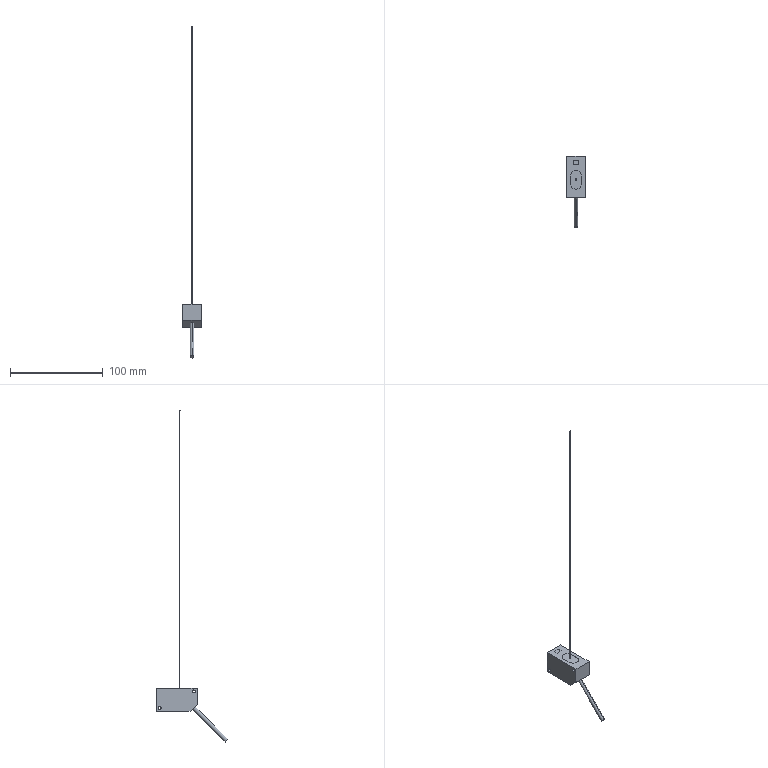Part | STEP file | hg-c series | 1 solid | 83 faces | box 20 x 76.982 x 357.882 mm | volume 21957 mm3 | plane 62 | cylinder 21 | commonest cylinder face diameters 1 x11 3.2 x4 4.1 x2 6.22 x2 12 x2